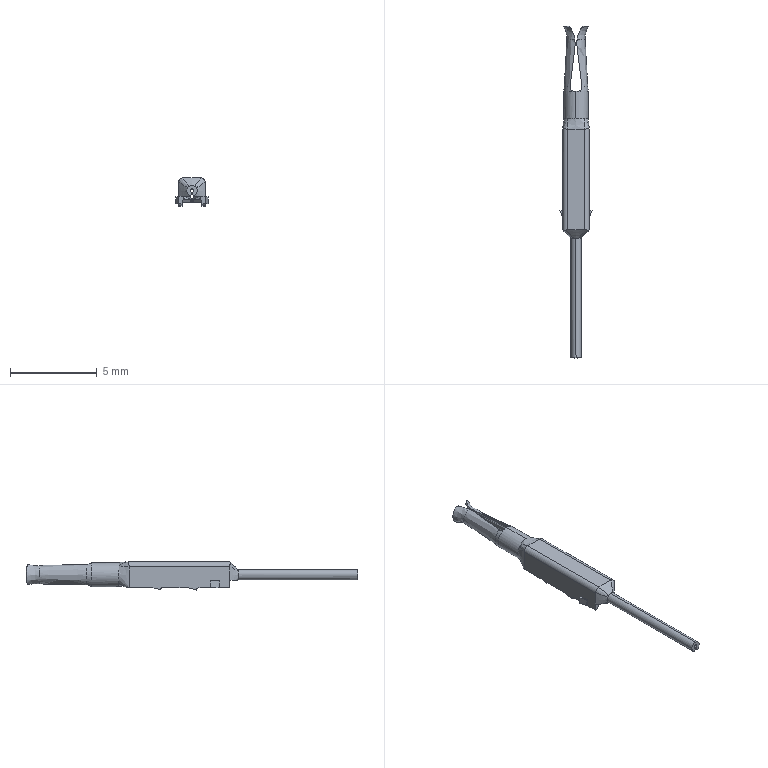Part | STEP file | CONTACT | 1 solid | 176 faces | box 1.85 x 19.165 x 1.65 mm | volume 9.871 mm3 | spline 68 | plane 66 | cylinder 32 | cone 10 | commonest cylinder face diameters 0.4 x6 3 x6 0.204 x4 0.26 x4 0.6 x4 0.396 x2